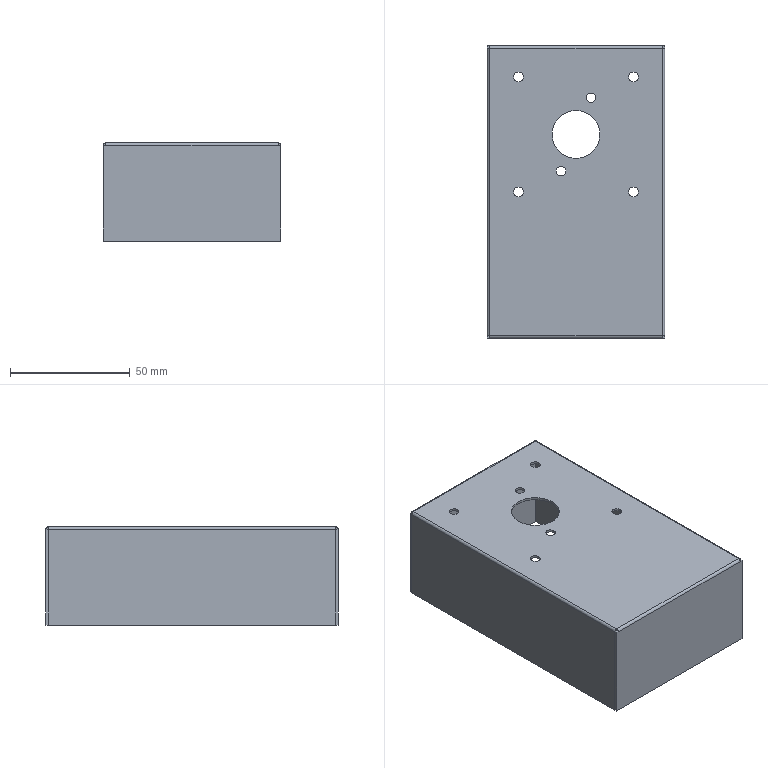Part | STEP file | Power knob mounting sheet metal | 1 solid | 56 faces | box 74 x 122 x 41 mm | volume 24069 mm3 | plane 34 | cylinder 22 | commonest cylinder face diameters 4 x12 0.02 x4 2.02 x4 20 x2